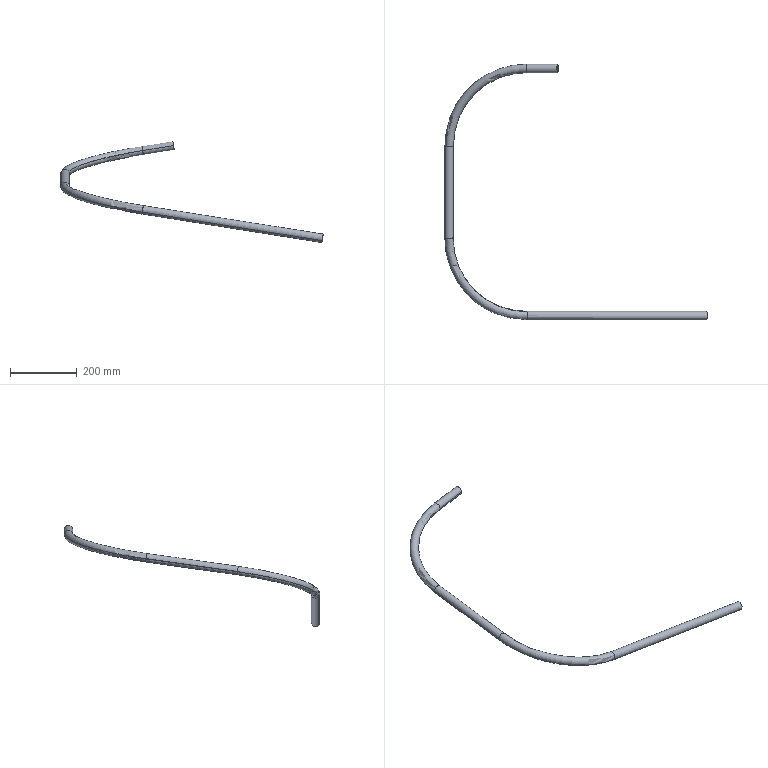Part | STEP file | 31E-01142WG10 | 1 solid | 22 faces | box 783.998 x 763.4 x 302.048 mm | volume 329314 mm3 | cylinder 12 | torus 8 | plane 2 | commonest cylinder face diameters 19.8 x6 25.4 x6
STEP:
#1=CARTESIAN_POINT('',(-1195.581,193.406,760.68));
#2=VERTEX_POINT('',#1);
#3=CARTESIAN_POINT('',(-1195.581,218.806,760.68));
#4=VERTEX_POINT('',#3);
#5=CARTESIAN_POINT('',(-1195.581,206.106,760.68));
#6=DIRECTION('',(-0.9877,0.,-0.1564));
#7=AXIS2_PLACEMENT_3D('',#5,#6,$);
#8=CIRCLE('',#7,12.7);
#9=EDGE_CURVE('',#2,#4,#8,.T.);
#10=ORIENTED_EDGE('',*,*,#9,.T.);
#11=CARTESIAN_POINT('',(-1287.732,218.806,746.085));
#12=VERTEX_POINT('',#11);
#13=CARTESIAN_POINT('',(-1241.656,218.806,753.382));
#14=DIRECTION('',(-0.9877,0.,-0.1564));
#15=VECTOR('',#14,1.);
#16=LINE('',#13,#15);
#17=EDGE_CURVE('',#12,#4,#16,.F.);
#18=ORIENTED_EDGE('',*,*,#17,.F.);
#19=CARTESIAN_POINT('',(-1287.732,193.406,746.085));
#20=VERTEX_POINT('',#19);
#21=CARTESIAN_POINT('',(-1287.732,206.106,746.085));
#22=DIRECTION('',(-0.9877,0.,-0.1564));
#23=AXIS2_PLACEMENT_3D('',#21,#22,$);
#24=CIRCLE('',#23,12.7);
#25=EDGE_CURVE('',#20,#12,#24,.T.);
#26=ORIENTED_EDGE('',*,*,#25,.F.);
#27=CARTESIAN_POINT('',(-1241.656,193.406,753.382));
#28=DIRECTION('',(-0.9877,0.,-0.1564));
#29=VECTOR('',#28,1.);
#30=LINE('',#27,#29);
#31=EDGE_CURVE('',#20,#2,#30,.F.);
#32=ORIENTED_EDGE('',*,*,#31,.T.);
#33=EDGE_LOOP('',(#10,#18,#26,#32));
#34=FACE_OUTER_BOUND('',#33,.T.);
#35=CARTESIAN_POINT('',(-1241.656,206.106,753.382));
#36=DIRECTION('',(-0.9877,0.,-0.1564));
#37=DIRECTION('',(0.,-1.,0.));
#38=AXIS2_PLACEMENT_3D('',#35,#36,#37);
#39=CYLINDRICAL_SURFACE('',#38,12.7);
#40=ADVANCED_FACE('',(#34),#39,.T.);
#41=CARTESIAN_POINT('',(-1195.581,206.106,760.68));
#42=DIRECTION('',(-0.9877,0.,-0.1564));
#43=AXIS2_PLACEMENT_3D('',#41,#42,$);
#44=CIRCLE('',#43,12.7);
#45=EDGE_CURVE('',#4,#2,#44,.T.);
#46=ORIENTED_EDGE('',*,*,#45,.T.);
#47=ORIENTED_EDGE('',*,*,#31,.F.);
#48=CARTESIAN_POINT('',(-1287.732,206.106,746.085));
#49=DIRECTION('',(-0.9877,0.,-0.1564));
#50=AXIS2_PLACEMENT_3D('',#48,#49,$);
#51=CIRCLE('',#50,12.7);
#52=EDGE_CURVE('',#12,#20,#51,.T.);
#53=ORIENTED_EDGE('',*,*,#52,.F.);
#54=ORIENTED_EDGE('',*,*,#17,.T.);
#55=EDGE_LOOP('',(#46,#47,#53,#54));
#56=FACE_OUTER_BOUND('',#55,.T.);
#57=CARTESIAN_POINT('',(-1241.656,206.106,753.382));
#58=DIRECTION('',(-0.9877,0.,-0.1564));
#59=DIRECTION('',(0.,1.,0.));
#60=AXIS2_PLACEMENT_3D('',#57,#58,#59);
#61=CYLINDRICAL_SURFACE('',#60,12.7);
#62=ADVANCED_FACE('',(#56),#61,.T.);
#63=CARTESIAN_POINT('',(-1507.514,-26.826,680.323));
#64=VERTEX_POINT('',#63);
#65=CARTESIAN_POINT('',(-1282.84,-31.855,715.201));
#66=DIRECTION('',(-0.1549,-0.1375,0.9783));
#67=AXIS2_PLACEMENT_3D('',#65,#66,$);
#68=CIRCLE('',#67,227.421);
#69=EDGE_CURVE('',#20,#64,#68,.T.);
#70=ORIENTED_EDGE('',*,*,#69,.F.);
#71=ORIENTED_EDGE('',*,*,#25,.T.);
#72=CARTESIAN_POINT('',(-1531.828,-25.79,673.048));
#73=VERTEX_POINT('',#72);
#74=CARTESIAN_POINT('',(-1282.299,-31.375,711.785));
#75=DIRECTION('',(-0.1549,-0.1375,0.9783));
#76=AXIS2_PLACEMENT_3D('',#74,#75,$);
#77=CIRCLE('',#76,252.579);
#78=EDGE_CURVE('',#12,#73,#77,.T.);
#79=ORIENTED_EDGE('',*,*,#78,.T.);
#80=CARTESIAN_POINT('',(-1519.671,-26.308,676.685));
#81=DIRECTION('',(0.0005446,0.9903,0.1393));
#82=AXIS2_PLACEMENT_3D('',#80,#81,$);
#83=CIRCLE('',#82,12.7);
#84=EDGE_CURVE('',#64,#73,#83,.F.);
#85=ORIENTED_EDGE('',*,*,#84,.F.);
#86=EDGE_LOOP('',(#70,#71,#79,#85));
#87=FACE_OUTER_BOUND('',#86,.T.);
#88=CARTESIAN_POINT('',(-1282.569,-31.615,713.493));
#89=DIRECTION('',(-0.1549,-0.1375,0.9783));
#90=DIRECTION('',(-0.02151,0.9905,0.1358));
#91=AXIS2_PLACEMENT_3D('',#88,#89,#90);
#92=TOROIDAL_SURFACE('',#91,240.,12.7);
#93=ADVANCED_FACE('',(#87),#92,.T.);
#94=ORIENTED_EDGE('',*,*,#45,.F.);
#95=ORIENTED_EDGE('',*,*,#9,.F.);
#96=EDGE_LOOP('',(#94,#95));
#97=FACE_OUTER_BOUND('',#96,.T.);
#98=CARTESIAN_POINT('',(-1195.581,216.006,760.68));
#99=VERTEX_POINT('',#98);
#100=CARTESIAN_POINT('',(-1195.581,196.206,760.68));
#101=VERTEX_POINT('',#100);
#102=CARTESIAN_POINT('',(-1195.581,206.106,760.68));
#103=DIRECTION('',(0.9877,0.,0.1564));
#104=AXIS2_PLACEMENT_3D('',#102,#103,$);
#105=CIRCLE('',#104,9.9);
#106=EDGE_CURVE('',#99,#101,#105,.F.);
#107=ORIENTED_EDGE('',*,*,#106,.T.);
#108=CARTESIAN_POINT('',(-1195.581,206.106,760.68));
#109=DIRECTION('',(0.9877,0.,0.1564));
#110=AXIS2_PLACEMENT_3D('',#108,#109,$);
#111=CIRCLE('',#110,9.9);
#112=EDGE_CURVE('',#101,#99,#111,.F.);
#113=ORIENTED_EDGE('',*,*,#112,.T.);
#114=EDGE_LOOP('',(#107,#113));
#115=FACE_BOUND('',#114,.T.);
#116=CARTESIAN_POINT('',(-1195.581,206.106,760.68));
#117=DIRECTION('',(0.9877,0.,0.1564));
#118=DIRECTION('',(0.,1.,0.));
#119=AXIS2_PLACEMENT_3D('',#116,#117,#118);
#120=PLANE('',#119);
#121=ADVANCED_FACE('',(#97,#115),#120,.T.);
#122=ORIENTED_EDGE('',*,*,#78,.F.);
#123=ORIENTED_EDGE('',*,*,#52,.T.);
#124=ORIENTED_EDGE('',*,*,#69,.T.);
#125=CARTESIAN_POINT('',(-1519.671,-26.308,676.685));
#126=DIRECTION('',(0.0005446,0.9903,0.1393));
#127=AXIS2_PLACEMENT_3D('',#125,#126,$);
#128=CIRCLE('',#127,12.7);
#129=EDGE_CURVE('',#73,#64,#128,.F.);
#130=ORIENTED_EDGE('',*,*,#129,.F.);
#131=EDGE_LOOP('',(#122,#123,#124,#130));
#132=FACE_OUTER_BOUND('',#131,.T.);
#133=CARTESIAN_POINT('',(-1282.569,-31.615,713.493));
#134=DIRECTION('',(-0.1549,-0.1375,0.9783));
#135=DIRECTION('',(-0.02151,0.9905,0.1358));
#136=AXIS2_PLACEMENT_3D('',#133,#134,#135);
#137=TOROIDAL_SURFACE('',#136,240.,12.7);
#138=ADVANCED_FACE('',(#132),#137,.T.);
#139=CARTESIAN_POINT('',(-1507.664,-299.748,641.943));
#140=VERTEX_POINT('',#139);
#141=CARTESIAN_POINT('',(-1507.589,-163.287,661.133));
#142=DIRECTION('',(-0.0005446,-0.9903,-0.1393));
#143=VECTOR('',#142,1.);
#144=LINE('',#141,#143);
#145=EDGE_CURVE('',#64,#140,#144,.T.);
#146=ORIENTED_EDGE('',*,*,#145,.F.);
#147=ORIENTED_EDGE('',*,*,#84,.T.);
#148=CARTESIAN_POINT('',(-1531.978,-298.711,634.668));
#149=VERTEX_POINT('',#148);
#150=CARTESIAN_POINT('',(-1531.903,-162.251,653.858));
#151=DIRECTION('',(-0.0005446,-0.9903,-0.1393));
#152=VECTOR('',#151,1.);
#153=LINE('',#150,#152);
#154=EDGE_CURVE('',#73,#149,#153,.T.);
#155=ORIENTED_EDGE('',*,*,#154,.T.);
#156=CARTESIAN_POINT('',(-1519.821,-299.229,638.305));
#157=DIRECTION('',(-0.0005446,-0.9903,-0.1393));
#158=AXIS2_PLACEMENT_3D('',#156,#157,$);
#159=CIRCLE('',#158,12.7);
#160=EDGE_CURVE('',#140,#149,#159,.T.);
#161=ORIENTED_EDGE('',*,*,#160,.F.);
#162=EDGE_LOOP('',(#146,#147,#155,#161));
#163=FACE_OUTER_BOUND('',#162,.T.);
#164=CARTESIAN_POINT('',(-1519.746,-162.769,657.495));
#165=DIRECTION('',(-0.0005446,-0.9903,-0.1393));
#166=DIRECTION('',(0.9572,-0.0408,0.2864));
#167=AXIS2_PLACEMENT_3D('',#164,#165,#166);
#168=CYLINDRICAL_SURFACE('',#167,12.7);
#169=ADVANCED_FACE('',(#163),#168,.T.);
#170=CARTESIAN_POINT('',(-1287.732,196.206,746.085));
#171=VERTEX_POINT('',#170);
#172=CARTESIAN_POINT('',(-1241.656,196.206,753.382));
#173=DIRECTION('',(-0.9877,0.,-0.1564));
#174=VECTOR('',#173,1.);
#175=LINE('',#172,#174);
#176=EDGE_CURVE('',#171,#101,#175,.F.);
#177=ORIENTED_EDGE('',*,*,#176,.F.);
#178=CARTESIAN_POINT('',(-1287.732,216.006,746.085));
#179=VERTEX_POINT('',#178);
#180=CARTESIAN_POINT('',(-1287.732,206.106,746.085));
#181=DIRECTION('',(-0.9877,0.,-0.1564));
#182=AXIS2_PLACEMENT_3D('',#180,#181,$);
#183=CIRCLE('',#182,9.9);
#184=EDGE_CURVE('',#171,#179,#183,.T.);
#185=ORIENTED_EDGE('',*,*,#184,.T.);
#186=CARTESIAN_POINT('',(-1241.656,216.006,753.382));
#187=DIRECTION('',(-0.9877,0.,-0.1564));
#188=VECTOR('',#187,1.);
#189=LINE('',#186,#188);
#190=EDGE_CURVE('',#179,#99,#189,.F.);
#191=ORIENTED_EDGE('',*,*,#190,.T.);
#192=ORIENTED_EDGE('',*,*,#112,.F.);
#193=EDGE_LOOP('',(#177,#185,#191,#192));
#194=FACE_OUTER_BOUND('',#193,.T.);
#195=CARTESIAN_POINT('',(-1241.656,206.106,753.382));
#196=DIRECTION('',(-0.9877,0.,-0.1564));
#197=DIRECTION('',(0.,-1.,0.));
#198=AXIS2_PLACEMENT_3D('',#195,#196,#197);
#199=CYLINDRICAL_SURFACE('',#198,9.9);
#200=ADVANCED_FACE('',(#194),#199,.F.);
#201=ORIENTED_EDGE('',*,*,#190,.F.);
#202=CARTESIAN_POINT('',(-1287.732,206.106,746.085));
#203=DIRECTION('',(-0.9877,0.,-0.1564));
#204=AXIS2_PLACEMENT_3D('',#202,#203,$);
#205=CIRCLE('',#204,9.9);
#206=EDGE_CURVE('',#179,#171,#205,.T.);
#207=ORIENTED_EDGE('',*,*,#206,.T.);
#208=ORIENTED_EDGE('',*,*,#176,.T.);
#209=ORIENTED_EDGE('',*,*,#106,.F.);
#210=EDGE_LOOP('',(#201,#207,#208,#209));
#211=FACE_OUTER_BOUND('',#210,.T.);
#212=CARTESIAN_POINT('',(-1241.656,206.106,753.382));
#213=DIRECTION('',(-0.9877,0.,-0.1564));
#214=DIRECTION('',(0.,1.,0.));
#215=AXIS2_PLACEMENT_3D('',#212,#213,#214);
#216=CYLINDRICAL_SURFACE('',#215,9.9);
#217=ADVANCED_FACE('',(#211),#216,.F.);
#218=ORIENTED_EDGE('',*,*,#154,.F.);
#219=ORIENTED_EDGE('',*,*,#129,.T.);
#220=ORIENTED_EDGE('',*,*,#145,.T.);
#221=CARTESIAN_POINT('',(-1519.821,-299.229,638.305));
#222=DIRECTION('',(-0.0005446,-0.9903,-0.1393));
#223=AXIS2_PLACEMENT_3D('',#221,#222,$);
#224=CIRCLE('',#223,12.7);
#225=EDGE_CURVE('',#149,#140,#224,.T.);
#226=ORIENTED_EDGE('',*,*,#225,.F.);
#227=EDGE_LOOP('',(#218,#219,#220,#226));
#228=FACE_OUTER_BOUND('',#227,.T.);
#229=CARTESIAN_POINT('',(-1519.746,-162.769,657.495));
#230=DIRECTION('',(-0.0005446,-0.9903,-0.1393));
#231=DIRECTION('',(-0.9572,0.0408,-0.2864));
#232=AXIS2_PLACEMENT_3D('',#229,#230,#231);
#233=CYLINDRICAL_SURFACE('',#232,12.7);
#234=ADVANCED_FACE('',(#228),#233,.T.);
#235=CARTESIAN_POINT('',(-1286.787,-521.321,575.78));
#236=VERTEX_POINT('',#235);
#237=CARTESIAN_POINT('',(-1281.865,-294.938,606.856));
#238=DIRECTION('',(0.1549,-0.1377,0.9783));
#239=AXIS2_PLACEMENT_3D('',#237,#238,$);
#240=CIRCLE('',#239,228.559);
#241=EDGE_CURVE('',#140,#236,#240,.T.);
#242=ORIENTED_EDGE('',*,*,#241,.F.);
#243=ORIENTED_EDGE('',*,*,#160,.T.);
#244=CARTESIAN_POINT('',(-1288.988,-542.467,561.882));
#245=VERTEX_POINT('',#244);
#246=CARTESIAN_POINT('',(-1283.574,-293.42,596.069));
#247=DIRECTION('',(0.1549,-0.1377,0.9783));
#248=AXIS2_PLACEMENT_3D('',#246,#247,$);
#249=CIRCLE('',#248,251.441);
#250=EDGE_CURVE('',#149,#245,#249,.T.);
#251=ORIENTED_EDGE('',*,*,#250,.T.);
#252=CARTESIAN_POINT('',(-1287.888,-531.894,568.831));
#253=DIRECTION('',(-0.9877,0.,0.1564));
#254=AXIS2_PLACEMENT_3D('',#252,#253,$);
#255=CIRCLE('',#254,12.7);
#256=EDGE_CURVE('',#236,#245,#255,.F.);
#257=ORIENTED_EDGE('',*,*,#256,.F.);
#258=EDGE_LOOP('',(#242,#243,#251,#257));
#259=FACE_OUTER_BOUND('',#258,.T.);
#260=CARTESIAN_POINT('',(-1282.719,-294.179,601.463));
#261=DIRECTION('',(0.1549,-0.1377,0.9783));
#262=DIRECTION('',(-0.9879,-0.02104,0.1535));
#263=AXIS2_PLACEMENT_3D('',#260,#261,#262);
#264=TOROIDAL_SURFACE('',#263,240.,12.7);
#265=ADVANCED_FACE('',(#259),#264,.T.);
#266=CARTESIAN_POINT('',(-1510.194,-26.712,679.521));
#267=VERTEX_POINT('',#266);
#268=CARTESIAN_POINT('',(-1529.147,-25.904,673.85));
#269=VERTEX_POINT('',#268);
#270=CARTESIAN_POINT('',(-1519.671,-26.308,676.685));
#271=DIRECTION('',(0.0005446,0.9903,0.1393));
#272=AXIS2_PLACEMENT_3D('',#270,#271,$);
#273=CIRCLE('',#272,9.9);
#274=EDGE_CURVE('',#267,#269,#273,.F.);
#275=ORIENTED_EDGE('',*,*,#274,.T.);
#276=CARTESIAN_POINT('',(-1282.359,-31.427,712.161));
#277=DIRECTION('',(-0.1549,-0.1375,0.9783));
#278=AXIS2_PLACEMENT_3D('',#276,#277,$);
#279=CIRCLE('',#278,249.806);
#280=EDGE_CURVE('',#179,#269,#279,.T.);
#281=ORIENTED_EDGE('',*,*,#280,.F.);
#282=ORIENTED_EDGE('',*,*,#184,.F.);
#283=CARTESIAN_POINT('',(-1282.78,-31.802,714.824));
#284=DIRECTION('',(-0.1549,-0.1375,0.9783));
#285=AXIS2_PLACEMENT_3D('',#283,#284,$);
#286=CIRCLE('',#285,230.194);
#287=EDGE_CURVE('',#171,#267,#286,.T.);
#288=ORIENTED_EDGE('',*,*,#287,.T.);
#289=EDGE_LOOP('',(#275,#281,#282,#288));
#290=FACE_OUTER_BOUND('',#289,.T.);
#291=CARTESIAN_POINT('',(-1282.569,-31.615,713.493));
#292=DIRECTION('',(-0.1549,-0.1375,0.9783));
#293=DIRECTION('',(-0.02151,0.9905,0.1358));
#294=AXIS2_PLACEMENT_3D('',#291,#292,#293);
#295=TOROIDAL_SURFACE('',#294,240.,9.9);
#296=ADVANCED_FACE('',(#290),#295,.F.);
#297=CARTESIAN_POINT('',(-1519.671,-26.308,676.685));
#298=DIRECTION('',(0.0005446,0.9903,0.1393));
#299=AXIS2_PLACEMENT_3D('',#297,#298,$);
#300=CIRCLE('',#299,9.9);
#301=EDGE_CURVE('',#269,#267,#300,.F.);
#302=ORIENTED_EDGE('',*,*,#301,.T.);
#303=ORIENTED_EDGE('',*,*,#287,.F.);
#304=ORIENTED_EDGE('',*,*,#206,.F.);
#305=ORIENTED_EDGE('',*,*,#280,.T.);
#306=EDGE_LOOP('',(#302,#303,#304,#305));
#307=FACE_OUTER_BOUND('',#306,.T.);
#308=CARTESIAN_POINT('',(-1282.569,-31.615,713.493));
#309=DIRECTION('',(-0.1549,-0.1375,0.9783));
#310=DIRECTION('',(-0.02151,0.9905,0.1358));
#311=AXIS2_PLACEMENT_3D('',#308,#309,#310);
#312=TOROIDAL_SURFACE('',#311,240.,9.9);
#313=ADVANCED_FACE('',(#307),#312,.F.);
#314=ORIENTED_EDGE('',*,*,#250,.F.);
#315=ORIENTED_EDGE('',*,*,#225,.T.);
#316=ORIENTED_EDGE('',*,*,#241,.T.);
#317=CARTESIAN_POINT('',(-1287.888,-531.894,568.831));
#318=DIRECTION('',(-0.9877,0.,0.1564));
#319=AXIS2_PLACEMENT_3D('',#317,#318,$);
#320=CIRCLE('',#319,12.7);
#321=EDGE_CURVE('',#245,#236,#320,.F.);
#322=ORIENTED_EDGE('',*,*,#321,.F.);
#323=EDGE_LOOP('',(#314,#315,#316,#322));
#324=FACE_OUTER_BOUND('',#323,.T.);
#325=CARTESIAN_POINT('',(-1282.719,-294.179,601.463));
#326=DIRECTION('',(0.1549,-0.1377,0.9783));
#327=DIRECTION('',(-0.9879,-0.02104,0.1535));
#328=AXIS2_PLACEMENT_3D('',#325,#326,#327);
#329=TOROIDAL_SURFACE('',#328,240.,12.7);
#330=ADVANCED_FACE('',(#324),#329,.T.);
#331=ORIENTED_EDGE('',*,*,#256,.T.);
#332=CARTESIAN_POINT('',(-751.611,-542.467,476.769));
#333=VERTEX_POINT('',#332);
#334=CARTESIAN_POINT('',(-1020.3,-542.467,519.326));
#335=DIRECTION('',(0.9877,0.,-0.1564));
#336=VECTOR('',#335,1.);
#337=LINE('',#334,#336);
#338=EDGE_CURVE('',#333,#245,#337,.F.);
#339=ORIENTED_EDGE('',*,*,#338,.F.);
#340=CARTESIAN_POINT('',(-749.409,-521.321,490.668));
#341=VERTEX_POINT('',#340);
#342=CARTESIAN_POINT('',(-750.51,-531.894,483.719));
#343=DIRECTION('',(0.9877,0.,-0.1564));
#344=AXIS2_PLACEMENT_3D('',#342,#343,$);
#345=CIRCLE('',#344,12.7);
#346=EDGE_CURVE('',#341,#333,#345,.T.);
#347=ORIENTED_EDGE('',*,*,#346,.F.);
#348=CARTESIAN_POINT('',(-1018.098,-521.321,533.224));
#349=DIRECTION('',(0.9877,0.,-0.1564));
#350=VECTOR('',#349,1.);
#351=LINE('',#348,#350);
#352=EDGE_CURVE('',#341,#236,#351,.F.);
#353=ORIENTED_EDGE('',*,*,#352,.T.);
#354=EDGE_LOOP('',(#331,#339,#347,#353));
#355=FACE_OUTER_BOUND('',#354,.T.);
#356=CARTESIAN_POINT('',(-1019.199,-531.894,526.275));
#357=DIRECTION('',(0.9877,0.,-0.1564));
#358=DIRECTION('',(0.08667,0.8325,0.5472));
#359=AXIS2_PLACEMENT_3D('',#356,#357,#358);
#360=CYLINDRICAL_SURFACE('',#359,12.7);
#361=ADVANCED_FACE('',(#355),#360,.T.);
#362=CARTESIAN_POINT('',(-1510.344,-299.633,641.141));
#363=VERTEX_POINT('',#362);
#364=CARTESIAN_POINT('',(-1529.298,-298.826,635.469));
#365=VERTEX_POINT('',#364);
#366=CARTESIAN_POINT('',(-1519.821,-299.229,638.305));
#367=DIRECTION('',(-0.0005446,-0.9903,-0.1393));
#368=AXIS2_PLACEMENT_3D('',#366,#367,$);
#369=CIRCLE('',#368,9.9);
#370=EDGE_CURVE('',#363,#365,#369,.T.);
#371=ORIENTED_EDGE('',*,*,#370,.T.);
#372=CARTESIAN_POINT('',(-1529.223,-162.365,654.66));
#373=DIRECTION('',(-0.0005446,-0.9903,-0.1393));
#374=VECTOR('',#373,1.);
#375=LINE('',#372,#374);
#376=EDGE_CURVE('',#269,#365,#375,.T.);
#377=ORIENTED_EDGE('',*,*,#376,.F.);
#378=ORIENTED_EDGE('',*,*,#274,.F.);
#379=CARTESIAN_POINT('',(-1510.269,-163.173,660.331));
#380=DIRECTION('',(-0.0005446,-0.9903,-0.1393));
#381=VECTOR('',#380,1.);
#382=LINE('',#379,#381);
#383=EDGE_CURVE('',#267,#363,#382,.T.);
#384=ORIENTED_EDGE('',*,*,#383,.T.);
#385=EDGE_LOOP('',(#371,#377,#378,#384));
#386=FACE_OUTER_BOUND('',#385,.T.);
#387=CARTESIAN_POINT('',(-1519.746,-162.769,657.495));
#388=DIRECTION('',(-0.0005446,-0.9903,-0.1393));
#389=DIRECTION('',(0.9572,-0.0408,0.2864));
#390=AXIS2_PLACEMENT_3D('',#387,#388,#389);
#391=CYLINDRICAL_SURFACE('',#390,9.9);
#392=ADVANCED_FACE('',(#386),#391,.F.);
#393=CARTESIAN_POINT('',(-1519.821,-299.229,638.305));
#394=DIRECTION('',(-0.0005446,-0.9903,-0.1393));
#395=AXIS2_PLACEMENT_3D('',#393,#394,$);
#396=CIRCLE('',#395,9.9);
#397=EDGE_CURVE('',#365,#363,#396,.T.);
#398=ORIENTED_EDGE('',*,*,#397,.T.);
#399=ORIENTED_EDGE('',*,*,#383,.F.);
#400=ORIENTED_EDGE('',*,*,#301,.F.);
#401=ORIENTED_EDGE('',*,*,#376,.T.);
#402=EDGE_LOOP('',(#398,#399,#400,#401));
#403=FACE_OUTER_BOUND('',#402,.T.);
#404=CARTESIAN_POINT('',(-1519.746,-162.769,657.495));
#405=DIRECTION('',(-0.0005446,-0.9903,-0.1393));
#406=DIRECTION('',(-0.9572,0.0408,-0.2864));
#407=AXIS2_PLACEMENT_3D('',#404,#405,#406);
#408=CYLINDRICAL_SURFACE('',#407,9.9);
#409=ADVANCED_FACE('',(#403),#408,.F.);
#410=ORIENTED_EDGE('',*,*,#321,.T.);
#411=ORIENTED_EDGE('',*,*,#352,.F.);
#412=CARTESIAN_POINT('',(-750.51,-531.894,483.719));
#413=DIRECTION('',(0.9877,0.,-0.1564));
#414=AXIS2_PLACEMENT_3D('',#412,#413,$);
#415=CIRCLE('',#414,12.7);
#416=EDGE_CURVE('',#333,#341,#415,.T.);
#417=ORIENTED_EDGE('',*,*,#416,.F.);
#418=ORIENTED_EDGE('',*,*,#338,.T.);
#419=EDGE_LOOP('',(#410,#411,#417,#418));
#420=FACE_OUTER_BOUND('',#419,.T.);
#421=CARTESIAN_POINT('',(-1019.199,-531.894,526.275));
#422=DIRECTION('',(0.9877,0.,-0.1564));
#423=DIRECTION('',(-0.08667,-0.8325,-0.5472));
#424=AXIS2_PLACEMENT_3D('',#421,#422,#423);
#425=CYLINDRICAL_SURFACE('',#424,12.7);
#426=ADVANCED_FACE('',(#420),#425,.T.);
#427=ORIENTED_EDGE('',*,*,#416,.T.);
#428=ORIENTED_EDGE('',*,*,#346,.T.);
#429=EDGE_LOOP('',(#427,#428));
#430=FACE_OUTER_BOUND('',#429,.T.);
#431=CARTESIAN_POINT('',(-749.652,-523.652,489.136));
#432=VERTEX_POINT('',#431);
#433=CARTESIAN_POINT('',(-751.368,-540.136,478.302));
#434=VERTEX_POINT('',#433);
#435=CARTESIAN_POINT('',(-750.51,-531.894,483.719));
#436=DIRECTION('',(0.9877,0.,-0.1564));
#437=AXIS2_PLACEMENT_3D('',#435,#436,$);
#438=CIRCLE('',#437,9.9);
#439=EDGE_CURVE('',#432,#434,#438,.T.);
#440=ORIENTED_EDGE('',*,*,#439,.F.);
#441=CARTESIAN_POINT('',(-750.51,-531.894,483.719));
#442=DIRECTION('',(0.9877,0.,-0.1564));
#443=AXIS2_PLACEMENT_3D('',#441,#442,$);
#444=CIRCLE('',#443,9.9);
#445=EDGE_CURVE('',#434,#432,#444,.T.);
#446=ORIENTED_EDGE('',*,*,#445,.F.);
#447=EDGE_LOOP('',(#440,#446));
#448=FACE_BOUND('',#447,.T.);
#449=CARTESIAN_POINT('',(-750.51,-531.894,483.719));
#450=DIRECTION('',(0.9877,0.,-0.1564));
#451=DIRECTION('',(0.,1.,0.));
#452=AXIS2_PLACEMENT_3D('',#449,#450,#451);
#453=PLANE('',#452);
#454=ADVANCED_FACE('',(#430,#448),#453,.T.);
#455=CARTESIAN_POINT('',(-1287.03,-523.652,574.248));
#456=VERTEX_POINT('',#455);
#457=CARTESIAN_POINT('',(-1288.746,-540.136,563.414));
#458=VERTEX_POINT('',#457);
#459=CARTESIAN_POINT('',(-1287.888,-531.894,568.831));
#460=DIRECTION('',(-0.9877,0.,0.1564));
#461=AXIS2_PLACEMENT_3D('',#459,#460,$);
#462=CIRCLE('',#461,9.9);
#463=EDGE_CURVE('',#456,#458,#462,.F.);
#464=ORIENTED_EDGE('',*,*,#463,.T.);
#465=CARTESIAN_POINT('',(-1283.385,-293.587,597.258));
#466=DIRECTION('',(0.1549,-0.1377,0.9783));
#467=AXIS2_PLACEMENT_3D('',#465,#466,$);
#468=CIRCLE('',#467,248.918);
#469=EDGE_CURVE('',#365,#458,#468,.T.);
#470=ORIENTED_EDGE('',*,*,#469,.F.);
#471=ORIENTED_EDGE('',*,*,#370,.F.);
#472=CARTESIAN_POINT('',(-1282.053,-294.77,605.667));
#473=DIRECTION('',(0.1549,-0.1377,0.9783));
#474=AXIS2_PLACEMENT_3D('',#472,#473,$);
#475=CIRCLE('',#474,231.082);
#476=EDGE_CURVE('',#363,#456,#475,.T.);
#477=ORIENTED_EDGE('',*,*,#476,.T.);
#478=EDGE_LOOP('',(#464,#470,#471,#477));
#479=FACE_OUTER_BOUND('',#478,.T.);
#480=CARTESIAN_POINT('',(-1282.719,-294.179,601.463));
#481=DIRECTION('',(0.1549,-0.1377,0.9783));
#482=DIRECTION('',(-0.9879,-0.02104,0.1535));
#483=AXIS2_PLACEMENT_3D('',#480,#481,#482);
#484=TOROIDAL_SURFACE('',#483,240.,9.9);
#485=ADVANCED_FACE('',(#479),#484,.F.);
#486=CARTESIAN_POINT('',(-1287.888,-531.894,568.831));
#487=DIRECTION('',(-0.9877,0.,0.1564));
#488=AXIS2_PLACEMENT_3D('',#486,#487,$);
#489=CIRCLE('',#488,9.9);
#490=EDGE_CURVE('',#458,#456,#489,.F.);
#491=ORIENTED_EDGE('',*,*,#490,.T.);
#492=ORIENTED_EDGE('',*,*,#476,.F.);
#493=ORIENTED_EDGE('',*,*,#397,.F.);
#494=ORIENTED_EDGE('',*,*,#469,.T.);
#495=EDGE_LOOP('',(#491,#492,#493,#494));
#496=FACE_OUTER_BOUND('',#495,.T.);
#497=CARTESIAN_POINT('',(-1282.719,-294.179,601.463));
#498=DIRECTION('',(0.1549,-0.1377,0.9783));
#499=DIRECTION('',(-0.9879,-0.02104,0.1535));
#500=AXIS2_PLACEMENT_3D('',#497,#498,#499);
#501=TOROIDAL_SURFACE('',#500,240.,9.9);
#502=ADVANCED_FACE('',(#496),#501,.F.);
#503=CARTESIAN_POINT('',(-1020.057,-540.136,520.858));
#504=DIRECTION('',(0.9877,0.,-0.1564));
#505=VECTOR('',#504,1.);
#506=LINE('',#503,#505);
#507=EDGE_CURVE('',#434,#458,#506,.F.);
#508=ORIENTED_EDGE('',*,*,#507,.F.);
#509=ORIENTED_EDGE('',*,*,#445,.T.);
#510=CARTESIAN_POINT('',(-1018.341,-523.652,531.692));
#511=DIRECTION('',(0.9877,0.,-0.1564));
#512=VECTOR('',#511,1.);
#513=LINE('',#510,#512);
#514=EDGE_CURVE('',#432,#456,#513,.F.);
#515=ORIENTED_EDGE('',*,*,#514,.T.);
#516=ORIENTED_EDGE('',*,*,#490,.F.);
#517=EDGE_LOOP('',(#508,#509,#515,#516));
#518=FACE_OUTER_BOUND('',#517,.T.);
#519=CARTESIAN_POINT('',(-1019.199,-531.894,526.275));
#520=DIRECTION('',(0.9877,0.,-0.1564));
#521=DIRECTION('',(-0.08667,-0.8325,-0.5472));
#522=AXIS2_PLACEMENT_3D('',#519,#520,#521);
#523=CYLINDRICAL_SURFACE('',#522,9.9);
#524=ADVANCED_FACE('',(#518),#523,.F.);
#525=ORIENTED_EDGE('',*,*,#514,.F.);
#526=ORIENTED_EDGE('',*,*,#439,.T.);
#527=ORIENTED_EDGE('',*,*,#507,.T.);
#528=ORIENTED_EDGE('',*,*,#463,.F.);
#529=EDGE_LOOP('',(#525,#526,#527,#528));
#530=FACE_OUTER_BOUND('',#529,.T.);
#531=CARTESIAN_POINT('',(-1019.199,-531.894,526.275));
#532=DIRECTION('',(0.9877,0.,-0.1564));
#533=DIRECTION('',(0.08667,0.8325,0.5472));
#534=AXIS2_PLACEMENT_3D('',#531,#532,#533);
#535=CYLINDRICAL_SURFACE('',#534,9.9);
#536=ADVANCED_FACE('',(#530),#535,.F.);
#537=CLOSED_SHELL('',(#40,#62,#93,#121,#138,#169,#200,#217,#234,#265,#296,#313,#330,#361,#392,#409,#426,#454,#485,#502,#524,#536));
#538=MANIFOLD_SOLID_BREP('',#537);
#539=(LENGTH_UNIT()NAMED_UNIT(*)SI_UNIT(.MILLI.,.METRE.));
#540=UNCERTAINTY_MEASURE_WITH_UNIT(LENGTH_MEASURE(0.005),#539,'','');
#541=(NAMED_UNIT(*)PLANE_ANGLE_UNIT()SI_UNIT($,.RADIAN.));
#542=(NAMED_UNIT(*)SI_UNIT($,.STERADIAN.)SOLID_ANGLE_UNIT());
#543=(GEOMETRIC_REPRESENTATION_CONTEXT(3)GLOBAL_UNCERTAINTY_ASSIGNED_CONTEXT((#540))GLOBAL_UNIT_ASSIGNED_CONTEXT((#539,#541,#542))REPRESENTATION_CONTEXT('',''));
#544=ADVANCED_BREP_SHAPE_REPRESENTATION('',(#538),#543);